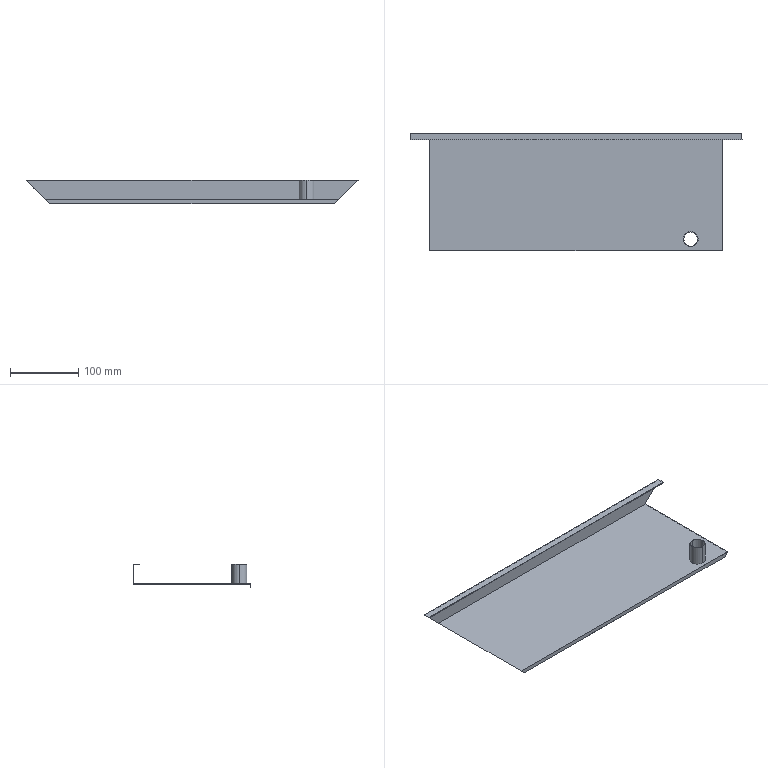Part | STEP file | 09-05 Inner side plate 2 | 1 solid | 17 faces | box 485 x 172 x 35 mm | volume 94551 mm3 | plane 13 | cylinder 4 | commonest cylinder face diameters 20 x2 22 x2
STEP:
#1=CARTESIAN_POINT('',(0.,0.,0.));
#2=DIRECTION('',(0.,0.,1.));
#3=DIRECTION('',(1.,0.,0.));
#4=AXIS2_PLACEMENT_3D('',#1,#2,#3);
#5=CARTESIAN_POINT('',(410.,6.,30.));
#6=VERTEX_POINT('',#5);
#7=CARTESIAN_POINT('',(410.,28.,30.));
#8=VERTEX_POINT('',#7);
#9=CARTESIAN_POINT('',(410.,17.,30.));
#10=DIRECTION('',(0.,0.,1.));
#11=DIRECTION('',(0.,1.,0.));
#12=AXIS2_PLACEMENT_3D('',#9,#10,#11);
#13=CIRCLE('',#12,11.);
#14=CARTESIAN_POINT('',(410.,17.,30.));
#15=DIRECTION('',(0.,0.,-1.));
#16=DIRECTION('',(0.,1.,0.));
#17=AXIS2_PLACEMENT_3D('',#14,#15,#16);
#18=CYLINDRICAL_SURFACE('',#17,11.);
#19=CARTESIAN_POINT('',(6.283,0.));
#20=DIRECTION('',(-1.,0.));
#21=VECTOR('',#20,1.);
#22=LINE('',#19,#21);
#23=(GEOMETRIC_REPRESENTATION_CONTEXT(2)PARAMETRIC_REPRESENTATION_CONTEXT()REPRESENTATION_CONTEXT('',''));
#24=DEFINITIONAL_REPRESENTATION('',(#22),#23);
#25=PCURVE('',#18,#24);
#26=CARTESIAN_POINT('',(398.868,5.868,30.));
#27=DIRECTION('',(0.,0.,1.));
#28=DIRECTION('',(1.,0.,0.));
#29=AXIS2_PLACEMENT_3D('',#26,#27,#28);
#30=PLANE('',#29);
#31=CARTESIAN_POINT('',(11.132,11.132));
#32=DIRECTION('',(0.,1.));
#33=AXIS2_PLACEMENT_2D('',#31,#32);
#34=CIRCLE('',#33,11.);
#35=(GEOMETRIC_REPRESENTATION_CONTEXT(2)PARAMETRIC_REPRESENTATION_CONTEXT()REPRESENTATION_CONTEXT('',''));
#36=DEFINITIONAL_REPRESENTATION('',(#34),#35);
#37=PCURVE('',#30,#36);
#38=SURFACE_CURVE('',#13,(#25,#37),.PCURVE_S1.);
#39=EDGE_CURVE('',#6,#8,#38,.T.);
#40=ORIENTED_EDGE('',*,*,#39,.F.);
#41=CARTESIAN_POINT('',(410.,6.,1.));
#42=VERTEX_POINT('',#41);
#43=CARTESIAN_POINT('',(410.,6.,30.));
#44=DIRECTION('',(0.,0.,-1.));
#45=VECTOR('',#44,1.);
#46=LINE('',#43,#45);
#47=CARTESIAN_POINT('',(3.142,0.));
#48=DIRECTION('',(0.,1.));
#49=VECTOR('',#48,1.);
#50=LINE('',#47,#49);
#51=(GEOMETRIC_REPRESENTATION_CONTEXT(2)PARAMETRIC_REPRESENTATION_CONTEXT()REPRESENTATION_CONTEXT('',''));
#52=DEFINITIONAL_REPRESENTATION('',(#50),#51);
#53=PCURVE('',#18,#52);
#54=CARTESIAN_POINT('',(410.,17.,30.));
#55=DIRECTION('',(0.,0.,-1.));
#56=DIRECTION('',(0.,1.,0.));
#57=AXIS2_PLACEMENT_3D('',#54,#55,#56);
#58=CYLINDRICAL_SURFACE('',#57,11.);
#59=CARTESIAN_POINT('',(3.142,0.));
#60=DIRECTION('',(0.,1.));
#61=VECTOR('',#60,1.);
#62=LINE('',#59,#61);
#63=(GEOMETRIC_REPRESENTATION_CONTEXT(2)PARAMETRIC_REPRESENTATION_CONTEXT()REPRESENTATION_CONTEXT('',''));
#64=DEFINITIONAL_REPRESENTATION('',(#62),#63);
#65=PCURVE('',#58,#64);
#66=SURFACE_CURVE('',#46,(#53,#65),.PCURVE_S1.);
#67=EDGE_CURVE('',#6,#42,#66,.T.);
#68=ORIENTED_EDGE('',*,*,#67,.T.);
#69=CARTESIAN_POINT('',(410.,28.,1.));
#70=VERTEX_POINT('',#69);
#71=CARTESIAN_POINT('',(410.,17.,1.));
#72=DIRECTION('',(0.,0.,-1.));
#73=DIRECTION('',(0.,1.,0.));
#74=AXIS2_PLACEMENT_3D('',#71,#72,#73);
#75=CIRCLE('',#74,11.);
#76=CARTESIAN_POINT('',(0.,29.));
#77=DIRECTION('',(1.,0.));
#78=VECTOR('',#77,1.);
#79=LINE('',#76,#78);
#80=(GEOMETRIC_REPRESENTATION_CONTEXT(2)PARAMETRIC_REPRESENTATION_CONTEXT()REPRESENTATION_CONTEXT('',''));
#81=DEFINITIONAL_REPRESENTATION('',(#79),#80);
#82=PCURVE('',#18,#81);
#83=CARTESIAN_POINT('',(29.,0.,1.));
#84=DIRECTION('',(0.,0.,-1.));
#85=DIRECTION('',(0.,1.,0.));
#86=AXIS2_PLACEMENT_3D('',#83,#84,#85);
#87=PLANE('',#86);
#88=CARTESIAN_POINT('',(17.,381.));
#89=DIRECTION('',(1.,0.));
#90=AXIS2_PLACEMENT_2D('',#88,#89);
#91=CIRCLE('',#90,11.);
#92=(GEOMETRIC_REPRESENTATION_CONTEXT(2)PARAMETRIC_REPRESENTATION_CONTEXT()REPRESENTATION_CONTEXT('',''));
#93=DEFINITIONAL_REPRESENTATION('',(#91),#92);
#94=PCURVE('',#87,#93);
#95=SURFACE_CURVE('',#75,(#82,#94),.PCURVE_S1.);
#96=EDGE_CURVE('',#70,#42,#95,.T.);
#97=ORIENTED_EDGE('',*,*,#96,.F.);
#98=CARTESIAN_POINT('',(410.,28.,30.));
#99=DIRECTION('',(0.,0.,-1.));
#100=VECTOR('',#99,1.);
#101=LINE('',#98,#100);
#102=CARTESIAN_POINT('',(0.,0.));
#103=DIRECTION('',(0.,1.));
#104=VECTOR('',#103,1.);
#105=LINE('',#102,#104);
#106=(GEOMETRIC_REPRESENTATION_CONTEXT(2)PARAMETRIC_REPRESENTATION_CONTEXT()REPRESENTATION_CONTEXT('',''));
#107=DEFINITIONAL_REPRESENTATION('',(#105),#106);
#108=PCURVE('',#18,#107);
#109=CARTESIAN_POINT('',(6.283,0.));
#110=DIRECTION('',(0.,1.));
#111=VECTOR('',#110,1.);
#112=LINE('',#109,#111);
#113=(GEOMETRIC_REPRESENTATION_CONTEXT(2)PARAMETRIC_REPRESENTATION_CONTEXT()REPRESENTATION_CONTEXT('',''));
#114=DEFINITIONAL_REPRESENTATION('',(#112),#113);
#115=PCURVE('',#58,#114);
#116=SURFACE_CURVE('',#101,(#108,#115),.PCURVE_S1.);
#117=EDGE_CURVE('',#8,#70,#116,.T.);
#118=ORIENTED_EDGE('',*,*,#117,.F.);
#119=EDGE_LOOP('',(#40,#68,#97,#118));
#120=FACE_BOUND('',#119,.T.);
#121=ADVANCED_FACE('',(#120),#18,.T.);
#122=CARTESIAN_POINT('',(400.,17.,30.));
#123=VERTEX_POINT('',#122);
#124=CARTESIAN_POINT('',(400.,17.,0.));
#125=VERTEX_POINT('',#124);
#126=CARTESIAN_POINT('',(400.,17.,30.));
#127=DIRECTION('',(0.,0.,-1.));
#128=VECTOR('',#127,1.);
#129=LINE('',#126,#128);
#130=CARTESIAN_POINT('',(410.,17.,30.));
#131=DIRECTION('',(0.,0.,-1.));
#132=DIRECTION('',(-1.,0.,0.));
#133=AXIS2_PLACEMENT_3D('',#130,#131,#132);
#134=CYLINDRICAL_SURFACE('',#133,10.);
#135=CARTESIAN_POINT('',(6.283,0.));
#136=DIRECTION('',(0.,1.));
#137=VECTOR('',#136,1.);
#138=LINE('',#135,#137);
#139=(GEOMETRIC_REPRESENTATION_CONTEXT(2)PARAMETRIC_REPRESENTATION_CONTEXT()REPRESENTATION_CONTEXT('',''));
#140=DEFINITIONAL_REPRESENTATION('',(#138),#139);
#141=PCURVE('',#134,#140);
#142=CARTESIAN_POINT('',(410.,17.,30.));
#143=DIRECTION('',(0.,0.,-1.));
#144=DIRECTION('',(-1.,0.,0.));
#145=AXIS2_PLACEMENT_3D('',#142,#143,#144);
#146=CYLINDRICAL_SURFACE('',#145,10.);
#147=CARTESIAN_POINT('',(0.,0.));
#148=DIRECTION('',(0.,1.));
#149=VECTOR('',#148,1.);
#150=LINE('',#147,#149);
#151=(GEOMETRIC_REPRESENTATION_CONTEXT(2)PARAMETRIC_REPRESENTATION_CONTEXT()REPRESENTATION_CONTEXT('',''));
#152=DEFINITIONAL_REPRESENTATION('',(#150),#151);
#153=PCURVE('',#146,#152);
#154=SURFACE_CURVE('',#129,(#141,#153),.PCURVE_S1.);
#155=EDGE_CURVE('',#123,#125,#154,.T.);
#156=ORIENTED_EDGE('',*,*,#155,.T.);
#157=CARTESIAN_POINT('',(420.,17.,0.));
#158=VERTEX_POINT('',#157);
#159=CARTESIAN_POINT('',(410.,17.,0.));
#160=DIRECTION('',(0.,0.,-1.));
#161=DIRECTION('',(-1.,0.,0.));
#162=AXIS2_PLACEMENT_3D('',#159,#160,#161);
#163=CIRCLE('',#162,10.);
#164=CARTESIAN_POINT('',(0.,30.));
#165=DIRECTION('',(1.,0.));
#166=VECTOR('',#165,1.);
#167=LINE('',#164,#166);
#168=(GEOMETRIC_REPRESENTATION_CONTEXT(2)PARAMETRIC_REPRESENTATION_CONTEXT()REPRESENTATION_CONTEXT('',''));
#169=DEFINITIONAL_REPRESENTATION('',(#167),#168);
#170=PCURVE('',#134,#169);
#171=CARTESIAN_POINT('',(30.,172.,0.));
#172=DIRECTION('',(0.,0.,1.));
#173=DIRECTION('',(0.,-1.,0.));
#174=AXIS2_PLACEMENT_3D('',#171,#172,#173);
#175=PLANE('',#174);
#176=CARTESIAN_POINT('',(155.,370.));
#177=CARTESIAN_POINT('',(137.679,370.));
#178=CARTESIAN_POINT('',(146.34,385.));
#179=CARTESIAN_POINT('',(155.,400.));
#180=CARTESIAN_POINT('',(163.66,385.));
#181=CARTESIAN_POINT('',(172.321,370.));
#182=CARTESIAN_POINT('',(155.,370.));
#183=(BOUNDED_CURVE()B_SPLINE_CURVE(2,(#176,#177,#178,#179,#180,#181,#182),.UNSPECIFIED.,.T.,.F.)B_SPLINE_CURVE_WITH_KNOTS((1,2,2,2,2,1),(-2.094,0.,2.094,4.189,6.283,8.378),.UNSPECIFIED.)CURVE()GEOMETRIC_REPRESENTATION_ITEM()RATIONAL_B_SPLINE_CURVE((1.,0.5,1.,0.5,1.,0.5,1.))REPRESENTATION_ITEM(''));
#184=(GEOMETRIC_REPRESENTATION_CONTEXT(2)PARAMETRIC_REPRESENTATION_CONTEXT()REPRESENTATION_CONTEXT('',''));
#185=DEFINITIONAL_REPRESENTATION('',(#183),#184);
#186=PCURVE('',#175,#185);
#187=SURFACE_CURVE('',#163,(#170,#186),.PCURVE_S1.);
#188=EDGE_CURVE('',#158,#125,#187,.T.);
#189=ORIENTED_EDGE('',*,*,#188,.F.);
#190=CARTESIAN_POINT('',(420.,17.,30.));
#191=VERTEX_POINT('',#190);
#192=CARTESIAN_POINT('',(420.,17.,30.));
#193=DIRECTION('',(0.,0.,-1.));
#194=VECTOR('',#193,1.);
#195=LINE('',#192,#194);
#196=CARTESIAN_POINT('',(3.142,0.));
#197=DIRECTION('',(0.,1.));
#198=VECTOR('',#197,1.);
#199=LINE('',#196,#198);
#200=(GEOMETRIC_REPRESENTATION_CONTEXT(2)PARAMETRIC_REPRESENTATION_CONTEXT()REPRESENTATION_CONTEXT('',''));
#201=DEFINITIONAL_REPRESENTATION('',(#199),#200);
#202=PCURVE('',#134,#201);
#203=CARTESIAN_POINT('',(3.142,0.));
#204=DIRECTION('',(0.,1.));
#205=VECTOR('',#204,1.);
#206=LINE('',#203,#205);
#207=(GEOMETRIC_REPRESENTATION_CONTEXT(2)PARAMETRIC_REPRESENTATION_CONTEXT()REPRESENTATION_CONTEXT('',''));
#208=DEFINITIONAL_REPRESENTATION('',(#206),#207);
#209=PCURVE('',#146,#208);
#210=SURFACE_CURVE('',#195,(#202,#209),.PCURVE_S1.);
#211=EDGE_CURVE('',#191,#158,#210,.T.);
#212=ORIENTED_EDGE('',*,*,#211,.F.);
#213=CARTESIAN_POINT('',(410.,17.,30.));
#214=DIRECTION('',(0.,0.,-1.));
#215=DIRECTION('',(-1.,0.,0.));
#216=AXIS2_PLACEMENT_3D('',#213,#214,#215);
#217=CIRCLE('',#216,10.);
#218=CARTESIAN_POINT('',(0.,0.));
#219=DIRECTION('',(1.,0.));
#220=VECTOR('',#219,1.);
#221=LINE('',#218,#220);
#222=(GEOMETRIC_REPRESENTATION_CONTEXT(2)PARAMETRIC_REPRESENTATION_CONTEXT()REPRESENTATION_CONTEXT('',''));
#223=DEFINITIONAL_REPRESENTATION('',(#221),#222);
#224=PCURVE('',#134,#223);
#225=CARTESIAN_POINT('',(1.132,11.132));
#226=CARTESIAN_POINT('',(1.132,28.453));
#227=CARTESIAN_POINT('',(16.132,19.792));
#228=CARTESIAN_POINT('',(31.132,11.132));
#229=CARTESIAN_POINT('',(16.132,2.472));
#230=CARTESIAN_POINT('',(1.132,-6.189));
#231=CARTESIAN_POINT('',(1.132,11.132));
#232=(BOUNDED_CURVE()B_SPLINE_CURVE(2,(#225,#226,#227,#228,#229,#230,#231),.UNSPECIFIED.,.T.,.F.)B_SPLINE_CURVE_WITH_KNOTS((1,2,2,2,2,1),(-2.094,0.,2.094,4.189,6.283,8.378),.UNSPECIFIED.)CURVE()GEOMETRIC_REPRESENTATION_ITEM()RATIONAL_B_SPLINE_CURVE((1.,0.5,1.,0.5,1.,0.5,1.))REPRESENTATION_ITEM(''));
#233=(GEOMETRIC_REPRESENTATION_CONTEXT(2)PARAMETRIC_REPRESENTATION_CONTEXT()REPRESENTATION_CONTEXT('',''));
#234=DEFINITIONAL_REPRESENTATION('',(#232),#233);
#235=PCURVE('',#30,#234);
#236=SURFACE_CURVE('',#217,(#224,#235),.PCURVE_S1.);
#237=EDGE_CURVE('',#191,#123,#236,.T.);
#238=ORIENTED_EDGE('',*,*,#237,.T.);
#239=EDGE_LOOP('',(#156,#189,#212,#238));
#240=FACE_BOUND('',#239,.F.);
#241=ADVANCED_FACE('',(#240),#134,.F.);
#242=ORIENTED_EDGE('',*,*,#67,.F.);
#243=CARTESIAN_POINT('',(410.,17.,30.));
#244=DIRECTION('',(0.,0.,1.));
#245=DIRECTION('',(0.,1.,0.));
#246=AXIS2_PLACEMENT_3D('',#243,#244,#245);
#247=CIRCLE('',#246,11.);
#248=CARTESIAN_POINT('',(6.283,0.));
#249=DIRECTION('',(-1.,0.));
#250=VECTOR('',#249,1.);
#251=LINE('',#248,#250);
#252=(GEOMETRIC_REPRESENTATION_CONTEXT(2)PARAMETRIC_REPRESENTATION_CONTEXT()REPRESENTATION_CONTEXT('',''));
#253=DEFINITIONAL_REPRESENTATION('',(#251),#252);
#254=PCURVE('',#58,#253);
#255=CARTESIAN_POINT('',(11.132,11.132));
#256=DIRECTION('',(0.,1.));
#257=AXIS2_PLACEMENT_2D('',#255,#256);
#258=CIRCLE('',#257,11.);
#259=(GEOMETRIC_REPRESENTATION_CONTEXT(2)PARAMETRIC_REPRESENTATION_CONTEXT()REPRESENTATION_CONTEXT('',''));
#260=DEFINITIONAL_REPRESENTATION('',(#258),#259);
#261=PCURVE('',#30,#260);
#262=SURFACE_CURVE('',#247,(#254,#261),.PCURVE_S1.);
#263=EDGE_CURVE('',#8,#6,#262,.T.);
#264=ORIENTED_EDGE('',*,*,#263,.F.);
#265=ORIENTED_EDGE('',*,*,#117,.T.);
#266=CARTESIAN_POINT('',(410.,17.,1.));
#267=DIRECTION('',(0.,0.,-1.));
#268=DIRECTION('',(0.,1.,0.));
#269=AXIS2_PLACEMENT_3D('',#266,#267,#268);
#270=CIRCLE('',#269,11.);
#271=CARTESIAN_POINT('',(0.,29.));
#272=DIRECTION('',(1.,0.));
#273=VECTOR('',#272,1.);
#274=LINE('',#271,#273);
#275=(GEOMETRIC_REPRESENTATION_CONTEXT(2)PARAMETRIC_REPRESENTATION_CONTEXT()REPRESENTATION_CONTEXT('',''));
#276=DEFINITIONAL_REPRESENTATION('',(#274),#275);
#277=PCURVE('',#58,#276);
#278=CARTESIAN_POINT('',(17.,381.));
#279=DIRECTION('',(1.,0.));
#280=AXIS2_PLACEMENT_2D('',#278,#279);
#281=CIRCLE('',#280,11.);
#282=(GEOMETRIC_REPRESENTATION_CONTEXT(2)PARAMETRIC_REPRESENTATION_CONTEXT()REPRESENTATION_CONTEXT('',''));
#283=DEFINITIONAL_REPRESENTATION('',(#281),#282);
#284=PCURVE('',#87,#283);
#285=SURFACE_CURVE('',#270,(#277,#284),.PCURVE_S1.);
#286=EDGE_CURVE('',#42,#70,#285,.T.);
#287=ORIENTED_EDGE('',*,*,#286,.F.);
#288=EDGE_LOOP('',(#242,#264,#265,#287));
#289=FACE_BOUND('',#288,.T.);
#290=ADVANCED_FACE('',(#289),#58,.T.);
#291=CARTESIAN_POINT('',(410.,17.,30.));
#292=DIRECTION('',(0.,0.,-1.));
#293=DIRECTION('',(-1.,0.,0.));
#294=AXIS2_PLACEMENT_3D('',#291,#292,#293);
#295=CIRCLE('',#294,10.);
#296=CARTESIAN_POINT('',(1.132,11.132));
#297=CARTESIAN_POINT('',(1.132,28.453));
#298=CARTESIAN_POINT('',(16.132,19.792));
#299=CARTESIAN_POINT('',(31.132,11.132));
#300=CARTESIAN_POINT('',(16.132,2.472));
#301=CARTESIAN_POINT('',(1.132,-6.189));
#302=CARTESIAN_POINT('',(1.132,11.132));
#303=(BOUNDED_CURVE()B_SPLINE_CURVE(2,(#296,#297,#298,#299,#300,#301,#302),.UNSPECIFIED.,.T.,.F.)B_SPLINE_CURVE_WITH_KNOTS((1,2,2,2,2,1),(-2.094,0.,2.094,4.189,6.283,8.378),.UNSPECIFIED.)CURVE()GEOMETRIC_REPRESENTATION_ITEM()RATIONAL_B_SPLINE_CURVE((1.,0.5,1.,0.5,1.,0.5,1.))REPRESENTATION_ITEM(''));
#304=(GEOMETRIC_REPRESENTATION_CONTEXT(2)PARAMETRIC_REPRESENTATION_CONTEXT()REPRESENTATION_CONTEXT('',''));
#305=DEFINITIONAL_REPRESENTATION('',(#303),#304);
#306=PCURVE('',#30,#305);
#307=CARTESIAN_POINT('',(0.,0.));
#308=DIRECTION('',(1.,0.));
#309=VECTOR('',#308,1.);
#310=LINE('',#307,#309);
#311=(GEOMETRIC_REPRESENTATION_CONTEXT(2)PARAMETRIC_REPRESENTATION_CONTEXT()REPRESENTATION_CONTEXT('',''));
#312=DEFINITIONAL_REPRESENTATION('',(#310),#311);
#313=PCURVE('',#146,#312);
#314=SURFACE_CURVE('',#295,(#306,#313),.PCURVE_S1.);
#315=EDGE_CURVE('',#123,#191,#314,.T.);
#316=ORIENTED_EDGE('',*,*,#315,.T.);
#317=ORIENTED_EDGE('',*,*,#237,.T.);
#318=EDGE_LOOP('',(#316,#317));
#319=FACE_BOUND('',#318,.T.);
#320=ORIENTED_EDGE('',*,*,#263,.T.);
#321=ORIENTED_EDGE('',*,*,#39,.T.);
#322=EDGE_LOOP('',(#320,#321));
#323=FACE_BOUND('',#322,.T.);
#324=ADVANCED_FACE('',(#319,#323),#30,.T.);
#325=ORIENTED_EDGE('',*,*,#96,.T.);
#326=ORIENTED_EDGE('',*,*,#286,.T.);
#327=EDGE_LOOP('',(#325,#326));
#328=FACE_BOUND('',#327,.T.);
#329=CARTESIAN_POINT('',(456.,171.,1.));
#330=VERTEX_POINT('',#329);
#331=CARTESIAN_POINT('',(456.,0.,1.));
#332=VERTEX_POINT('',#331);
#333=CARTESIAN_POINT('',(456.,85.5,1.));
#334=DIRECTION('',(0.,-1.,0.));
#335=VECTOR('',#334,1.);
#336=LINE('',#333,#335);
#337=CARTESIAN_POINT('',(85.5,427.));
#338=DIRECTION('',(-1.,0.));
#339=VECTOR('',#338,1.);
#340=LINE('',#337,#339);
#341=(GEOMETRIC_REPRESENTATION_CONTEXT(2)PARAMETRIC_REPRESENTATION_CONTEXT()REPRESENTATION_CONTEXT('',''));
#342=DEFINITIONAL_REPRESENTATION('',(#340),#341);
#343=PCURVE('',#87,#342);
#344=CARTESIAN_POINT('',(450.,0.,-5.));
#345=DIRECTION('',(-0.7071,0.,0.7071));
#346=DIRECTION('',(0.7071,0.,0.7071));
#347=AXIS2_PLACEMENT_3D('',#344,#345,#346);
#348=PLANE('',#347);
#349=CARTESIAN_POINT('',(8.485,85.5));
#350=DIRECTION('',(0.,-1.));
#351=VECTOR('',#350,1.);
#352=LINE('',#349,#351);
#353=(GEOMETRIC_REPRESENTATION_CONTEXT(2)PARAMETRIC_REPRESENTATION_CONTEXT()REPRESENTATION_CONTEXT('',''));
#354=DEFINITIONAL_REPRESENTATION('',(#352),#353);
#355=PCURVE('',#348,#354);
#356=SURFACE_CURVE('',#336,(#343,#355),.PCURVE_S1.);
#357=EDGE_CURVE('',#330,#332,#356,.T.);
#358=ORIENTED_EDGE('',*,*,#357,.F.);
#359=CARTESIAN_POINT('',(29.,171.,1.));
#360=VERTEX_POINT('',#359);
#361=CARTESIAN_POINT('',(242.5,171.,1.));
#362=DIRECTION('',(1.,0.,0.));
#363=VECTOR('',#362,1.);
#364=LINE('',#361,#363);
#365=CARTESIAN_POINT('',(171.,213.5));
#366=DIRECTION('',(0.,1.));
#367=VECTOR('',#366,1.);
#368=LINE('',#365,#367);
#369=(GEOMETRIC_REPRESENTATION_CONTEXT(2)PARAMETRIC_REPRESENTATION_CONTEXT()REPRESENTATION_CONTEXT('',''));
#370=DEFINITIONAL_REPRESENTATION('',(#368),#369);
#371=PCURVE('',#87,#370);
#372=CARTESIAN_POINT('',(-1.898,171.,1.));
#373=DIRECTION('',(0.,1.,0.));
#374=DIRECTION('',(0.,0.,1.));
#375=AXIS2_PLACEMENT_3D('',#372,#373,#374);
#376=PLANE('',#375);
#377=CARTESIAN_POINT('',(0.,244.398));
#378=DIRECTION('',(0.,1.));
#379=VECTOR('',#378,1.);
#380=LINE('',#377,#379);
#381=(GEOMETRIC_REPRESENTATION_CONTEXT(2)PARAMETRIC_REPRESENTATION_CONTEXT()REPRESENTATION_CONTEXT('',''));
#382=DEFINITIONAL_REPRESENTATION('',(#380),#381);
#383=PCURVE('',#376,#382);
#384=SURFACE_CURVE('',#364,(#371,#383),.PCURVE_S1.);
#385=EDGE_CURVE('',#360,#330,#384,.T.);
#386=ORIENTED_EDGE('',*,*,#385,.F.);
#387=CARTESIAN_POINT('',(29.,0.,1.));
#388=VERTEX_POINT('',#387);
#389=CARTESIAN_POINT('',(29.,85.5,1.));
#390=DIRECTION('',(0.,1.,0.));
#391=VECTOR('',#390,1.);
#392=LINE('',#389,#391);
#393=CARTESIAN_POINT('',(85.5,0.));
#394=DIRECTION('',(1.,0.));
#395=VECTOR('',#394,1.);
#396=LINE('',#393,#395);
#397=(GEOMETRIC_REPRESENTATION_CONTEXT(2)PARAMETRIC_REPRESENTATION_CONTEXT()REPRESENTATION_CONTEXT('',''));
#398=DEFINITIONAL_REPRESENTATION('',(#396),#397);
#399=PCURVE('',#87,#398);
#400=CARTESIAN_POINT('',(0.,0.,30.));
#401=DIRECTION('',(0.7071,0.,0.7071));
#402=DIRECTION('',(0.7071,0.,-0.7071));
#403=AXIS2_PLACEMENT_3D('',#400,#401,#402);
#404=PLANE('',#403);
#405=CARTESIAN_POINT('',(41.012,85.5));
#406=DIRECTION('',(0.,1.));
#407=VECTOR('',#406,1.);
#408=LINE('',#405,#407);
#409=(GEOMETRIC_REPRESENTATION_CONTEXT(2)PARAMETRIC_REPRESENTATION_CONTEXT()REPRESENTATION_CONTEXT('',''));
#410=DEFINITIONAL_REPRESENTATION('',(#408),#409);
#411=PCURVE('',#404,#410);
#412=SURFACE_CURVE('',#392,(#399,#411),.PCURVE_S1.);
#413=EDGE_CURVE('',#388,#360,#412,.T.);
#414=ORIENTED_EDGE('',*,*,#413,.F.);
#415=CARTESIAN_POINT('',(242.5,0.,1.));
#416=DIRECTION('',(-1.,0.,0.));
#417=VECTOR('',#416,1.);
#418=LINE('',#415,#417);
#419=CARTESIAN_POINT('',(0.,213.5));
#420=DIRECTION('',(0.,-1.));
#421=VECTOR('',#420,1.);
#422=LINE('',#419,#421);
#423=(GEOMETRIC_REPRESENTATION_CONTEXT(2)PARAMETRIC_REPRESENTATION_CONTEXT()REPRESENTATION_CONTEXT('',''));
#424=DEFINITIONAL_REPRESENTATION('',(#422),#423);
#425=PCURVE('',#87,#424);
#426=CARTESIAN_POINT('',(26.438,0.,-5.));
#427=DIRECTION('',(0.,1.,0.));
#428=DIRECTION('',(0.,0.,1.));
#429=AXIS2_PLACEMENT_3D('',#426,#427,#428);
#430=PLANE('',#429);
#431=CARTESIAN_POINT('',(6.,216.062));
#432=DIRECTION('',(0.,-1.));
#433=VECTOR('',#432,1.);
#434=LINE('',#431,#433);
#435=(GEOMETRIC_REPRESENTATION_CONTEXT(2)PARAMETRIC_REPRESENTATION_CONTEXT()REPRESENTATION_CONTEXT('',''));
#436=DEFINITIONAL_REPRESENTATION('',(#434),#435);
#437=PCURVE('',#430,#436);
#438=SURFACE_CURVE('',#418,(#425,#437),.PCURVE_S1.);
#439=EDGE_CURVE('',#332,#388,#438,.T.);
#440=ORIENTED_EDGE('',*,*,#439,.F.);
#441=EDGE_LOOP('',(#358,#386,#414,#440));
#442=FACE_BOUND('',#441,.T.);
#443=ADVANCED_FACE('',(#328,#442),#87,.F.);
#444=CARTESIAN_POINT('',(410.,17.,0.));
#445=DIRECTION('',(0.,0.,-1.));
#446=DIRECTION('',(-1.,0.,0.));
#447=AXIS2_PLACEMENT_3D('',#444,#445,#446);
#448=CIRCLE('',#447,10.);
#449=CARTESIAN_POINT('',(0.,30.));
#450=DIRECTION('',(1.,0.));
#451=VECTOR('',#450,1.);
#452=LINE('',#449,#451);
#453=(GEOMETRIC_REPRESENTATION_CONTEXT(2)PARAMETRIC_REPRESENTATION_CONTEXT()REPRESENTATION_CONTEXT('',''));
#454=DEFINITIONAL_REPRESENTATION('',(#452),#453);
#455=PCURVE('',#146,#454);
#456=CARTESIAN_POINT('',(155.,370.));
#457=CARTESIAN_POINT('',(137.679,370.));
#458=CARTESIAN_POINT('',(146.34,385.));
#459=CARTESIAN_POINT('',(155.,400.));
#460=CARTESIAN_POINT('',(163.66,385.));
#461=CARTESIAN_POINT('',(172.321,370.));
#462=CARTESIAN_POINT('',(155.,370.));
#463=(BOUNDED_CURVE()B_SPLINE_CURVE(2,(#456,#457,#458,#459,#460,#461,#462),.UNSPECIFIED.,.T.,.F.)B_SPLINE_CURVE_WITH_KNOTS((1,2,2,2,2,1),(-2.094,0.,2.094,4.189,6.283,8.378),.UNSPECIFIED.)CURVE()GEOMETRIC_REPRESENTATION_ITEM()RATIONAL_B_SPLINE_CURVE((1.,0.5,1.,0.5,1.,0.5,1.))REPRESENTATION_ITEM(''));
#464=(GEOMETRIC_REPRESENTATION_CONTEXT(2)PARAMETRIC_REPRESENTATION_CONTEXT()REPRESENTATION_CONTEXT('',''));
#465=DEFINITIONAL_REPRESENTATION('',(#463),#464);
#466=PCURVE('',#175,#465);
#467=SURFACE_CURVE('',#448,(#455,#466),.PCURVE_S1.);
#468=EDGE_CURVE('',#125,#158,#467,.T.);
#469=ORIENTED_EDGE('',*,*,#468,.F.);
#470=ORIENTED_EDGE('',*,*,#155,.F.);
#471=ORIENTED_EDGE('',*,*,#315,.T.);
#472=ORIENTED_EDGE('',*,*,#211,.T.);
#473=EDGE_LOOP('',(#469,#470,#471,#472));
#474=FACE_BOUND('',#473,.F.);
#475=ADVANCED_FACE('',(#474),#146,.F.);
#476=CARTESIAN_POINT('',(450.,0.,-5.));
#477=VERTEX_POINT('',#476);
#478=CARTESIAN_POINT('',(450.,0.,-5.));
#479=DIRECTION('',(-0.7071,0.,-0.7071));
#480=VECTOR('',#479,1.);
#481=LINE('',#478,#480);
#482=CARTESIAN_POINT('',(0.,423.562));
#483=DIRECTION('',(-0.7071,-0.7071));
#484=VECTOR('',#483,1.);
#485=LINE('',#482,#484);
#486=(GEOMETRIC_REPRESENTATION_CONTEXT(2)PARAMETRIC_REPRESENTATION_CONTEXT()REPRESENTATION_CONTEXT('',''));
#487=DEFINITIONAL_REPRESENTATION('',(#485),#486);
#488=PCURVE('',#430,#487);
#489=CARTESIAN_POINT('',(0.,0.));
#490=DIRECTION('',(-1.,0.));
#491=VECTOR('',#490,1.);
#492=LINE('',#489,#491);
#493=(GEOMETRIC_REPRESENTATION_CONTEXT(2)PARAMETRIC_REPRESENTATION_CONTEXT()REPRESENTATION_CONTEXT('',''));
#494=DEFINITIONAL_REPRESENTATION('',(#492),#493);
#495=PCURVE('',#348,#494);
#496=SURFACE_CURVE('',#481,(#488,#495),.PCURVE_S1.);
#497=EDGE_CURVE('',#332,#477,#496,.T.);
#498=ORIENTED_EDGE('',*,*,#497,.F.);
#499=ORIENTED_EDGE('',*,*,#439,.T.);
#500=CARTESIAN_POINT('',(35.,0.,-5.));
#501=VERTEX_POINT('',#500);
#502=CARTESIAN_POINT('',(0.,0.,30.));
#503=DIRECTION('',(-0.7071,0.,0.7071));
#504=VECTOR('',#503,1.);
#505=LINE('',#502,#504);
#506=CARTESIAN_POINT('',(35.,-26.438));
#507=DIRECTION('',(0.7071,-0.7071));
#508=VECTOR('',#507,1.);
#509=LINE('',#506,#508);
#510=(GEOMETRIC_REPRESENTATION_CONTEXT(2)PARAMETRIC_REPRESENTATION_CONTEXT()REPRESENTATION_CONTEXT('',''));
#511=DEFINITIONAL_REPRESENTATION('',(#509),#510);
#512=PCURVE('',#430,#511);
#513=CARTESIAN_POINT('',(0.,0.));
#514=DIRECTION('',(-1.,0.));
#515=VECTOR('',#514,1.);
#516=LINE('',#513,#515);
#517=(GEOMETRIC_REPRESENTATION_CONTEXT(2)PARAMETRIC_REPRESENTATION_CONTEXT()REPRESENTATION_CONTEXT('',''));
#518=DEFINITIONAL_REPRESENTATION('',(#516),#517);
#519=PCURVE('',#404,#518);
#520=SURFACE_CURVE('',#505,(#512,#519),.PCURVE_S1.);
#521=EDGE_CURVE('',#501,#388,#520,.T.);
#522=ORIENTED_EDGE('',*,*,#521,.F.);
#523=CARTESIAN_POINT('',(242.5,0.,-5.));
#524=DIRECTION('',(-1.,0.,0.));
#525=VECTOR('',#524,1.);
#526=LINE('',#523,#525);
#527=CARTESIAN_POINT('',(0.,216.062));
#528=DIRECTION('',(0.,-1.));
#529=VECTOR('',#528,1.);
#530=LINE('',#527,#529);
#531=(GEOMETRIC_REPRESENTATION_CONTEXT(2)PARAMETRIC_REPRESENTATION_CONTEXT()REPRESENTATION_CONTEXT('',''));
#532=DEFINITIONAL_REPRESENTATION('',(#530),#531);
#533=PCURVE('',#430,#532);
#534=CARTESIAN_POINT('',(35.,0.,-5.));
#535=DIRECTION('',(0.,0.,1.));
#536=DIRECTION('',(1.,0.,0.));
#537=AXIS2_PLACEMENT_3D('',#534,#535,#536);
#538=PLANE('',#537);
#539=CARTESIAN_POINT('',(207.5,0.));
#540=DIRECTION('',(-1.,0.));
#541=VECTOR('',#540,1.);
#542=LINE('',#539,#541);
#543=(GEOMETRIC_REPRESENTATION_CONTEXT(2)PARAMETRIC_REPRESENTATION_CONTEXT()REPRESENTATION_CONTEXT('',''));
#544=DEFINITIONAL_REPRESENTATION('',(#542),#543);
#545=PCURVE('',#538,#544);
#546=SURFACE_CURVE('',#526,(#533,#545),.PCURVE_S1.);
#547=EDGE_CURVE('',#477,#501,#546,.T.);
#548=ORIENTED_EDGE('',*,*,#547,.F.);
#549=EDGE_LOOP('',(#498,#499,#522,#548));
#550=FACE_BOUND('',#549,.T.);
#551=ADVANCED_FACE('',(#550),#430,.F.);
#552=CARTESIAN_POINT('',(485.,172.,30.));
#553=VERTEX_POINT('',#552);
#554=CARTESIAN_POINT('',(455.,172.,0.000000001));
#555=VERTEX_POINT('',#554);
#556=CARTESIAN_POINT('',(467.5,172.,12.5));
#557=DIRECTION('',(-0.7071,0.,-0.7071));
#558=VECTOR('',#557,1.);
#559=LINE('',#556,#558);
#560=CARTESIAN_POINT('',(24.749,172.));
#561=DIRECTION('',(-1.,0.));
#562=VECTOR('',#561,1.);
#563=LINE('',#560,#562);
#564=(GEOMETRIC_REPRESENTATION_CONTEXT(2)PARAMETRIC_REPRESENTATION_CONTEXT()REPRESENTATION_CONTEXT('',''));
#565=DEFINITIONAL_REPRESENTATION('',(#563),#564);
#566=PCURVE('',#348,#565);
#567=CARTESIAN_POINT('',(-2.91,172.,30.));
#568=DIRECTION('',(0.,-1.,0.));
#569=DIRECTION('',(0.,0.,-1.));
#570=AXIS2_PLACEMENT_3D('',#567,#568,#569);
#571=PLANE('',#570);
#572=CARTESIAN_POINT('',(17.5,470.41));
#573=DIRECTION('',(0.7071,-0.7071));
#574=VECTOR('',#573,1.);
#575=LINE('',#572,#574);
#576=(GEOMETRIC_REPRESENTATION_CONTEXT(2)PARAMETRIC_REPRESENTATION_CONTEXT()REPRESENTATION_CONTEXT('',''));
#577=DEFINITIONAL_REPRESENTATION('',(#575),#576);
#578=PCURVE('',#571,#577);
#579=SURFACE_CURVE('',#559,(#566,#578),.PCURVE_S1.);
#580=EDGE_CURVE('',#553,#555,#579,.T.);
#581=ORIENTED_EDGE('',*,*,#580,.F.);
#582=CARTESIAN_POINT('',(485.,162.,30.));
#583=VERTEX_POINT('',#582);
#584=CARTESIAN_POINT('',(485.,86.,30.));
#585=DIRECTION('',(0.,1.,0.));
#586=VECTOR('',#585,1.);
#587=LINE('',#584,#586);
#588=CARTESIAN_POINT('',(49.497,86.));
#589=DIRECTION('',(0.,1.));
#590=VECTOR('',#589,1.);
#591=LINE('',#588,#590);
#592=(GEOMETRIC_REPRESENTATION_CONTEXT(2)PARAMETRIC_REPRESENTATION_CONTEXT()REPRESENTATION_CONTEXT('',''));
#593=DEFINITIONAL_REPRESENTATION('',(#591),#592);
#594=PCURVE('',#348,#593);
#595=CARTESIAN_POINT('',(0.,162.,30.));
#596=DIRECTION('',(0.,0.,-1.));
#597=DIRECTION('',(0.,1.,0.));
#598=AXIS2_PLACEMENT_3D('',#595,#596,#597);
#599=PLANE('',#598);
#600=CARTESIAN_POINT('',(-76.,485.));
#601=DIRECTION('',(1.,0.));
#602=VECTOR('',#601,1.);
#603=LINE('',#600,#602);
#604=(GEOMETRIC_REPRESENTATION_CONTEXT(2)PARAMETRIC_REPRESENTATION_CONTEXT()REPRESENTATION_CONTEXT('',''));
#605=DEFINITIONAL_REPRESENTATION('',(#603),#604);
#606=PCURVE('',#599,#605);
#607=SURFACE_CURVE('',#587,(#594,#606),.PCURVE_S1.);
#608=EDGE_CURVE('',#583,#553,#607,.T.);
#609=ORIENTED_EDGE('',*,*,#608,.F.);
#610=CARTESIAN_POINT('',(484.,162.,29.));
#611=VERTEX_POINT('',#610);
#612=CARTESIAN_POINT('',(450.,162.,-5.));
#613=DIRECTION('',(-0.7071,0.,-0.7071));
#614=VECTOR('',#613,1.);
#615=LINE('',#612,#614);
#616=CARTESIAN_POINT('',(0.,162.));
#617=DIRECTION('',(-1.,0.));
#618=VECTOR('',#617,1.);
#619=LINE('',#616,#618);
#620=(GEOMETRIC_REPRESENTATION_CONTEXT(2)PARAMETRIC_REPRESENTATION_CONTEXT()REPRESENTATION_CONTEXT('',''));
#621=DEFINITIONAL_REPRESENTATION('',(#619),#620);
#622=PCURVE('',#348,#621);
#623=CARTESIAN_POINT('',(-2.91,162.,29.));
#624=DIRECTION('',(0.,1.,0.));
#625=DIRECTION('',(0.,0.,1.));
#626=AXIS2_PLACEMENT_3D('',#623,#624,#625);
#627=PLANE('',#626);
#628=CARTESIAN_POINT('',(-34.,452.91));
#629=DIRECTION('',(-0.7071,-0.7071));
#630=VECTOR('',#629,1.);
#631=LINE('',#628,#630);
#632=(GEOMETRIC_REPRESENTATION_CONTEXT(2)PARAMETRIC_REPRESENTATION_CONTEXT()REPRESENTATION_CONTEXT('',''));
#633=DEFINITIONAL_REPRESENTATION('',(#631),#632);
#634=PCURVE('',#627,#633);
#635=SURFACE_CURVE('',#615,(#622,#634),.PCURVE_S1.);
#636=EDGE_CURVE('',#583,#611,#635,.T.);
#637=ORIENTED_EDGE('',*,*,#636,.T.);
#638=CARTESIAN_POINT('',(484.,171.,29.));
#639=VERTEX_POINT('',#638);
#640=CARTESIAN_POINT('',(484.,86.,29.));
#641=DIRECTION('',(0.,-1.,0.));
#642=VECTOR('',#641,1.);
#643=LINE('',#640,#642);
#644=CARTESIAN_POINT('',(48.083,86.));
#645=DIRECTION('',(0.,-1.));
#646=VECTOR('',#645,1.);
#647=LINE('',#644,#646);
#648=(GEOMETRIC_REPRESENTATION_CONTEXT(2)PARAMETRIC_REPRESENTATION_CONTEXT()REPRESENTATION_CONTEXT('',''));
#649=DEFINITIONAL_REPRESENTATION('',(#647),#648);
#650=PCURVE('',#348,#649);
#651=CARTESIAN_POINT('',(1.,162.,29.));
#652=DIRECTION('',(0.,0.,1.));
#653=DIRECTION('',(1.,0.,0.));
#654=AXIS2_PLACEMENT_3D('',#651,#652,#653);
#655=PLANE('',#654);
#656=CARTESIAN_POINT('',(483.,-76.));
#657=DIRECTION('',(0.,-1.));
#658=VECTOR('',#657,1.);
#659=LINE('',#656,#658);
#660=(GEOMETRIC_REPRESENTATION_CONTEXT(2)PARAMETRIC_REPRESENTATION_CONTEXT()REPRESENTATION_CONTEXT('',''));
#661=DEFINITIONAL_REPRESENTATION('',(#659),#660);
#662=PCURVE('',#655,#661);
#663=SURFACE_CURVE('',#643,(#650,#662),.PCURVE_S1.);
#664=EDGE_CURVE('',#639,#611,#663,.T.);
#665=ORIENTED_EDGE('',*,*,#664,.F.);
#666=CARTESIAN_POINT('',(467.5,171.,12.5));
#667=DIRECTION('',(0.7071,0.,0.7071));
#668=VECTOR('',#667,1.);
#669=LINE('',#666,#668);
#670=CARTESIAN_POINT('',(24.749,171.));
#671=DIRECTION('',(1.,0.));
#672=VECTOR('',#671,1.);
#673=LINE('',#670,#672);
#674=(GEOMETRIC_REPRESENTATION_CONTEXT(2)PARAMETRIC_REPRESENTATION_CONTEXT()REPRESENTATION_CONTEXT('',''));
#675=DEFINITIONAL_REPRESENTATION('',(#673),#674);
#676=PCURVE('',#348,#675);
#677=CARTESIAN_POINT('',(11.5,469.398));
#678=DIRECTION('',(0.7071,0.7071));
#679=VECTOR('',#678,1.);
#680=LINE('',#677,#679);
#681=(GEOMETRIC_REPRESENTATION_CONTEXT(2)PARAMETRIC_REPRESENTATION_CONTEXT()REPRESENTATION_CONTEXT('',''));
#682=DEFINITIONAL_REPRESENTATION('',(#680),#681);
#683=PCURVE('',#376,#682);
#684=SURFACE_CURVE('',#669,(#676,#683),.PCURVE_S1.);
#685=EDGE_CURVE('',#330,#639,#684,.T.);
#686=ORIENTED_EDGE('',*,*,#685,.F.);
#687=ORIENTED_EDGE('',*,*,#357,.T.);
#688=ORIENTED_EDGE('',*,*,#497,.T.);
#689=CARTESIAN_POINT('',(450.,1.,-5.));
#690=VERTEX_POINT('',#689);
#691=CARTESIAN_POINT('',(450.,86.,-5.));
#692=DIRECTION('',(0.,-1.,0.));
#693=VECTOR('',#692,1.);
#694=LINE('',#691,#693);
#695=CARTESIAN_POINT('',(0.,86.));
#696=DIRECTION('',(0.,-1.));
#697=VECTOR('',#696,1.);
#698=LINE('',#695,#697);
#699=(GEOMETRIC_REPRESENTATION_CONTEXT(2)PARAMETRIC_REPRESENTATION_CONTEXT()REPRESENTATION_CONTEXT('',''));
#700=DEFINITIONAL_REPRESENTATION('',(#698),#699);
#701=PCURVE('',#348,#700);
#702=CARTESIAN_POINT('',(415.,86.));
#703=DIRECTION('',(0.,-1.));
#704=VECTOR('',#703,1.);
#705=LINE('',#702,#704);
#706=(GEOMETRIC_REPRESENTATION_CONTEXT(2)PARAMETRIC_REPRESENTATION_CONTEXT()REPRESENTATION_CONTEXT('',''));
#707=DEFINITIONAL_REPRESENTATION('',(#705),#706);
#708=PCURVE('',#538,#707);
#709=SURFACE_CURVE('',#694,(#701,#708),.PCURVE_S1.);
#710=EDGE_CURVE('',#690,#477,#709,.T.);
#711=ORIENTED_EDGE('',*,*,#710,.F.);
#712=CARTESIAN_POINT('',(455.,1.,0.000000001));
#713=VERTEX_POINT('',#712);
#714=CARTESIAN_POINT('',(467.5,1.,12.5));
#715=DIRECTION('',(-0.7071,0.,-0.7071));
#716=VECTOR('',#715,1.);
#717=LINE('',#714,#716);
#718=CARTESIAN_POINT('',(24.749,1.));
#719=DIRECTION('',(-1.,0.));
#720=VECTOR('',#719,1.);
#721=LINE('',#718,#720);
#722=(GEOMETRIC_REPRESENTATION_CONTEXT(2)PARAMETRIC_REPRESENTATION_CONTEXT()REPRESENTATION_CONTEXT('',''));
#723=DEFINITIONAL_REPRESENTATION('',(#721),#722);
#724=PCURVE('',#348,#723);
#725=CARTESIAN_POINT('',(27.45,1.,0.));
#726=DIRECTION('',(0.,-1.,0.));
#727=DIRECTION('',(0.,0.,-1.));
#728=AXIS2_PLACEMENT_3D('',#725,#726,#727);
#729=PLANE('',#728);
#730=CARTESIAN_POINT('',(-12.5,440.05));
#731=DIRECTION('',(0.7071,-0.7071));
#732=VECTOR('',#731,1.);
#733=LINE('',#730,#732);
#734=(GEOMETRIC_REPRESENTATION_CONTEXT(2)PARAMETRIC_REPRESENTATION_CONTEXT()REPRESENTATION_CONTEXT('',''));
#735=DEFINITIONAL_REPRESENTATION('',(#733),#734);
#736=PCURVE('',#729,#735);
#737=SURFACE_CURVE('',#717,(#724,#736),.PCURVE_S1.);
#738=EDGE_CURVE('',#713,#690,#737,.T.);
#739=ORIENTED_EDGE('',*,*,#738,.F.);
#740=CARTESIAN_POINT('',(455.,86.,0.000000005));
#741=DIRECTION('',(0.,-1.,0.));
#742=VECTOR('',#741,1.);
#743=LINE('',#740,#742);
#744=CARTESIAN_POINT('',(7.071,86.));
#745=DIRECTION('',(0.,-1.));
#746=VECTOR('',#745,1.);
#747=LINE('',#744,#746);
#748=(GEOMETRIC_REPRESENTATION_CONTEXT(2)PARAMETRIC_REPRESENTATION_CONTEXT()REPRESENTATION_CONTEXT('',''));
#749=DEFINITIONAL_REPRESENTATION('',(#747),#748);
#750=PCURVE('',#348,#749);
#751=CARTESIAN_POINT('',(86.,425.));
#752=DIRECTION('',(1.,0.));
#753=VECTOR('',#752,1.);
#754=LINE('',#751,#753);
#755=(GEOMETRIC_REPRESENTATION_CONTEXT(2)PARAMETRIC_REPRESENTATION_CONTEXT()REPRESENTATION_CONTEXT('',''));
#756=DEFINITIONAL_REPRESENTATION('',(#754),#755);
#757=PCURVE('',#175,#756);
#758=SURFACE_CURVE('',#743,(#750,#757),.PCURVE_S1.);
#759=EDGE_CURVE('',#555,#713,#758,.T.);
#760=ORIENTED_EDGE('',*,*,#759,.F.);
#761=EDGE_LOOP('',(#581,#609,#637,#665,#686,#687,#688,#711,#739,#760));
#762=FACE_BOUND('',#761,.T.);
#763=ADVANCED_FACE('',(#762),#348,.F.);
#764=ORIENTED_EDGE('',*,*,#685,.T.);
#765=CARTESIAN_POINT('',(1.,171.,29.));
#766=VERTEX_POINT('',#765);
#767=CARTESIAN_POINT('',(242.5,171.,29.));
#768=DIRECTION('',(1.,0.,0.));
#769=VECTOR('',#768,1.);
#770=LINE('',#767,#769);
#771=CARTESIAN_POINT('',(28.,244.398));
#772=DIRECTION('',(0.,1.));
#773=VECTOR('',#772,1.);
#774=LINE('',#771,#773);
#775=(GEOMETRIC_REPRESENTATION_CONTEXT(2)PARAMETRIC_REPRESENTATION_CONTEXT()REPRESENTATION_CONTEXT('',''));
#776=DEFINITIONAL_REPRESENTATION('',(#774),#775);
#777=PCURVE('',#376,#776);
#778=CARTESIAN_POINT('',(241.5,9.));
#779=DIRECTION('',(1.,0.));
#780=VECTOR('',#779,1.);
#781=LINE('',#778,#780);
#782=(GEOMETRIC_REPRESENTATION_CONTEXT(2)PARAMETRIC_REPRESENTATION_CONTEXT()REPRESENTATION_CONTEXT('',''));
#783=DEFINITIONAL_REPRESENTATION('',(#781),#782);
#784=PCURVE('',#655,#783);
#785=SURFACE_CURVE('',#770,(#777,#784),.PCURVE_S1.);
#786=EDGE_CURVE('',#766,#639,#785,.T.);
#787=ORIENTED_EDGE('',*,*,#786,.F.);
#788=CARTESIAN_POINT('',(0.,171.,30.));
#789=DIRECTION('',(-0.7071,0.,0.7071));
#790=VECTOR('',#789,1.);
#791=LINE('',#788,#790);
#792=CARTESIAN_POINT('',(29.,1.898));
#793=DIRECTION('',(0.7071,-0.7071));
#794=VECTOR('',#793,1.);
#795=LINE('',#792,#794);
#796=(GEOMETRIC_REPRESENTATION_CONTEXT(2)PARAMETRIC_REPRESENTATION_CONTEXT()REPRESENTATION_CONTEXT('',''));
#797=DEFINITIONAL_REPRESENTATION('',(#795),#796);
#798=PCURVE('',#376,#797);
#799=CARTESIAN_POINT('',(0.,171.));
#800=DIRECTION('',(-1.,0.));
#801=VECTOR('',#800,1.);
#802=LINE('',#799,#801);
#803=(GEOMETRIC_REPRESENTATION_CONTEXT(2)PARAMETRIC_REPRESENTATION_CONTEXT()REPRESENTATION_CONTEXT('',''));
#804=DEFINITIONAL_REPRESENTATION('',(#802),#803);
#805=PCURVE('',#404,#804);
#806=SURFACE_CURVE('',#791,(#798,#805),.PCURVE_S1.);
#807=EDGE_CURVE('',#360,#766,#806,.T.);
#808=ORIENTED_EDGE('',*,*,#807,.F.);
#809=ORIENTED_EDGE('',*,*,#385,.T.);
#810=EDGE_LOOP('',(#764,#787,#808,#809));
#811=FACE_BOUND('',#810,.T.);
#812=ADVANCED_FACE('',(#811),#376,.F.);
#813=ORIENTED_EDGE('',*,*,#521,.T.);
#814=ORIENTED_EDGE('',*,*,#413,.T.);
#815=ORIENTED_EDGE('',*,*,#807,.T.);
#816=CARTESIAN_POINT('',(1.,162.,29.));
#817=VERTEX_POINT('',#816);
#818=CARTESIAN_POINT('',(1.,86.,29.));
#819=DIRECTION('',(0.,1.,0.));
#820=VECTOR('',#819,1.);
#821=LINE('',#818,#820);
#822=CARTESIAN_POINT('',(1.414,86.));
#823=DIRECTION('',(0.,1.));
#824=VECTOR('',#823,1.);
#825=LINE('',#822,#824);
#826=(GEOMETRIC_REPRESENTATION_CONTEXT(2)PARAMETRIC_REPRESENTATION_CONTEXT()REPRESENTATION_CONTEXT('',''));
#827=DEFINITIONAL_REPRESENTATION('',(#825),#826);
#828=PCURVE('',#404,#827);
#829=CARTESIAN_POINT('',(0.000000015,-76.));
#830=DIRECTION('',(0.,1.));
#831=VECTOR('',#830,1.);
#832=LINE('',#829,#831);
#833=(GEOMETRIC_REPRESENTATION_CONTEXT(2)PARAMETRIC_REPRESENTATION_CONTEXT()REPRESENTATION_CONTEXT('',''));
#834=DEFINITIONAL_REPRESENTATION('',(#832),#833);
#835=PCURVE('',#655,#834);
#836=SURFACE_CURVE('',#821,(#828,#835),.PCURVE_S1.);
#837=EDGE_CURVE('',#817,#766,#836,.T.);
#838=ORIENTED_EDGE('',*,*,#837,.F.);
#839=CARTESIAN_POINT('',(0.,162.,30.));
#840=VERTEX_POINT('',#839);
#841=CARTESIAN_POINT('',(0.,162.,30.));
#842=DIRECTION('',(-0.7071,0.,0.7071));
#843=VECTOR('',#842,1.);
#844=LINE('',#841,#843);
#845=CARTESIAN_POINT('',(0.,162.));
#846=DIRECTION('',(-1.,0.));
#847=VECTOR('',#846,1.);
#848=LINE('',#845,#847);
#849=(GEOMETRIC_REPRESENTATION_CONTEXT(2)PARAMETRIC_REPRESENTATION_CONTEXT()REPRESENTATION_CONTEXT('',''));
#850=DEFINITIONAL_REPRESENTATION('',(#848),#849);
#851=PCURVE('',#404,#850);
#852=CARTESIAN_POINT('',(1.,2.91));
#853=DIRECTION('',(0.7071,-0.7071));
#854=VECTOR('',#853,1.);
#855=LINE('',#852,#854);
#856=(GEOMETRIC_REPRESENTATION_CONTEXT(2)PARAMETRIC_REPRESENTATION_CONTEXT()REPRESENTATION_CONTEXT('',''));
#857=DEFINITIONAL_REPRESENTATION('',(#855),#856);
#858=PCURVE('',#627,#857);
#859=SURFACE_CURVE('',#844,(#851,#858),.PCURVE_S1.);
#860=EDGE_CURVE('',#817,#840,#859,.T.);
#861=ORIENTED_EDGE('',*,*,#860,.T.);
#862=CARTESIAN_POINT('',(0.00000006,172.,30.));
#863=VERTEX_POINT('',#862);
#864=CARTESIAN_POINT('',(0.,86.,30.));
#865=DIRECTION('',(0.,-1.,0.));
#866=VECTOR('',#865,1.);
#867=LINE('',#864,#866);
#868=CARTESIAN_POINT('',(0.,86.));
#869=DIRECTION('',(0.,-1.));
#870=VECTOR('',#869,1.);
#871=LINE('',#868,#870);
#872=(GEOMETRIC_REPRESENTATION_CONTEXT(2)PARAMETRIC_REPRESENTATION_CONTEXT()REPRESENTATION_CONTEXT('',''));
#873=DEFINITIONAL_REPRESENTATION('',(#871),#872);
#874=PCURVE('',#404,#873);
#875=CARTESIAN_POINT('',(-76.,0.));
#876=DIRECTION('',(-1.,0.));
#877=VECTOR('',#876,1.);
#878=LINE('',#875,#877);
#879=(GEOMETRIC_REPRESENTATION_CONTEXT(2)PARAMETRIC_REPRESENTATION_CONTEXT()REPRESENTATION_CONTEXT('',''));
#880=DEFINITIONAL_REPRESENTATION('',(#878),#879);
#881=PCURVE('',#599,#880);
#882=SURFACE_CURVE('',#867,(#874,#881),.PCURVE_S1.);
#883=EDGE_CURVE('',#863,#840,#882,.T.);
#884=ORIENTED_EDGE('',*,*,#883,.F.);
#885=CARTESIAN_POINT('',(30.,172.,0.000000001));
#886=VERTEX_POINT('',#885);
#887=CARTESIAN_POINT('',(17.5,172.,12.5));
#888=DIRECTION('',(-0.7071,0.,0.7071));
#889=VECTOR('',#888,1.);
#890=LINE('',#887,#889);
#891=CARTESIAN_POINT('',(24.749,172.));
#892=DIRECTION('',(-1.,0.));
#893=VECTOR('',#892,1.);
#894=LINE('',#891,#893);
#895=(GEOMETRIC_REPRESENTATION_CONTEXT(2)PARAMETRIC_REPRESENTATION_CONTEXT()REPRESENTATION_CONTEXT('',''));
#896=DEFINITIONAL_REPRESENTATION('',(#894),#895);
#897=PCURVE('',#404,#896);
#898=CARTESIAN_POINT('',(17.5,20.41));
#899=DIRECTION('',(-0.7071,-0.7071));
#900=VECTOR('',#899,1.);
#901=LINE('',#898,#900);
#902=(GEOMETRIC_REPRESENTATION_CONTEXT(2)PARAMETRIC_REPRESENTATION_CONTEXT()REPRESENTATION_CONTEXT('',''));
#903=DEFINITIONAL_REPRESENTATION('',(#901),#902);
#904=PCURVE('',#571,#903);
#905=SURFACE_CURVE('',#890,(#897,#904),.PCURVE_S1.);
#906=EDGE_CURVE('',#886,#863,#905,.T.);
#907=ORIENTED_EDGE('',*,*,#906,.F.);
#908=CARTESIAN_POINT('',(30.,1.,0.000000001));
#909=VERTEX_POINT('',#908);
#910=CARTESIAN_POINT('',(30.,86.,0.000000005));
#911=DIRECTION('',(0.,1.,0.));
#912=VECTOR('',#911,1.);
#913=LINE('',#910,#912);
#914=CARTESIAN_POINT('',(42.426,86.));
#915=DIRECTION('',(0.,1.));
#916=VECTOR('',#915,1.);
#917=LINE('',#914,#916);
#918=(GEOMETRIC_REPRESENTATION_CONTEXT(2)PARAMETRIC_REPRESENTATION_CONTEXT()REPRESENTATION_CONTEXT('',''));
#919=DEFINITIONAL_REPRESENTATION('',(#917),#918);
#920=PCURVE('',#404,#919);
#921=CARTESIAN_POINT('',(86.,-0.000000005));
#922=DIRECTION('',(-1.,0.));
#923=VECTOR('',#922,1.);
#924=LINE('',#921,#923);
#925=(GEOMETRIC_REPRESENTATION_CONTEXT(2)PARAMETRIC_REPRESENTATION_CONTEXT()REPRESENTATION_CONTEXT('',''));
#926=DEFINITIONAL_REPRESENTATION('',(#924),#925);
#927=PCURVE('',#175,#926);
#928=SURFACE_CURVE('',#913,(#920,#927),.PCURVE_S1.);
#929=EDGE_CURVE('',#909,#886,#928,.T.);
#930=ORIENTED_EDGE('',*,*,#929,.F.);
#931=CARTESIAN_POINT('',(35.,1.,-5.));
#932=VERTEX_POINT('',#931);
#933=CARTESIAN_POINT('',(17.5,1.,12.5));
#934=DIRECTION('',(-0.7071,0.,0.7071));
#935=VECTOR('',#934,1.);
#936=LINE('',#933,#935);
#937=CARTESIAN_POINT('',(24.749,1.));
#938=DIRECTION('',(-1.,0.));
#939=VECTOR('',#938,1.);
#940=LINE('',#937,#939);
#941=(GEOMETRIC_REPRESENTATION_CONTEXT(2)PARAMETRIC_REPRESENTATION_CONTEXT()REPRESENTATION_CONTEXT('',''));
#942=DEFINITIONAL_REPRESENTATION('',(#940),#941);
#943=PCURVE('',#404,#942);
#944=CARTESIAN_POINT('',(-12.5,-9.95));
#945=DIRECTION('',(-0.7071,-0.7071));
#946=VECTOR('',#945,1.);
#947=LINE('',#944,#946);
#948=(GEOMETRIC_REPRESENTATION_CONTEXT(2)PARAMETRIC_REPRESENTATION_CONTEXT()REPRESENTATION_CONTEXT('',''));
#949=DEFINITIONAL_REPRESENTATION('',(#947),#948);
#950=PCURVE('',#729,#949);
#951=SURFACE_CURVE('',#936,(#943,#950),.PCURVE_S1.);
#952=EDGE_CURVE('',#932,#909,#951,.T.);
#953=ORIENTED_EDGE('',*,*,#952,.F.);
#954=CARTESIAN_POINT('',(35.,86.,-5.));
#955=DIRECTION('',(0.,1.,0.));
#956=VECTOR('',#955,1.);
#957=LINE('',#954,#956);
#958=CARTESIAN_POINT('',(49.497,86.));
#959=DIRECTION('',(0.,1.));
#960=VECTOR('',#959,1.);
#961=LINE('',#958,#960);
#962=(GEOMETRIC_REPRESENTATION_CONTEXT(2)PARAMETRIC_REPRESENTATION_CONTEXT()REPRESENTATION_CONTEXT('',''));
#963=DEFINITIONAL_REPRESENTATION('',(#961),#962);
#964=PCURVE('',#404,#963);
#965=CARTESIAN_POINT('',(0.,86.));
#966=DIRECTION('',(0.,1.));
#967=VECTOR('',#966,1.);
#968=LINE('',#965,#967);
#969=(GEOMETRIC_REPRESENTATION_CONTEXT(2)PARAMETRIC_REPRESENTATION_CONTEXT()REPRESENTATION_CONTEXT('',''));
#970=DEFINITIONAL_REPRESENTATION('',(#968),#969);
#971=PCURVE('',#538,#970);
#972=SURFACE_CURVE('',#957,(#964,#971),.PCURVE_S1.);
#973=EDGE_CURVE('',#501,#932,#972,.T.);
#974=ORIENTED_EDGE('',*,*,#973,.F.);
#975=EDGE_LOOP('',(#813,#814,#815,#838,#861,#884,#907,#930,#953,#974));
#976=FACE_BOUND('',#975,.T.);
#977=ADVANCED_FACE('',(#976),#404,.F.);
#978=ORIENTED_EDGE('',*,*,#468,.F.);
#979=ORIENTED_EDGE('',*,*,#188,.F.);
#980=EDGE_LOOP('',(#978,#979));
#981=FACE_BOUND('',#980,.T.);
#982=ORIENTED_EDGE('',*,*,#759,.T.);
#983=CARTESIAN_POINT('',(242.5,1.,0.));
#984=DIRECTION('',(1.,0.,0.));
#985=VECTOR('',#984,1.);
#986=LINE('',#983,#985);
#987=CARTESIAN_POINT('',(171.,212.5));
#988=DIRECTION('',(0.,1.));
#989=VECTOR('',#988,1.);
#990=LINE('',#987,#989);
#991=(GEOMETRIC_REPRESENTATION_CONTEXT(2)PARAMETRIC_REPRESENTATION_CONTEXT()REPRESENTATION_CONTEXT('',''));
#992=DEFINITIONAL_REPRESENTATION('',(#990),#991);
#993=PCURVE('',#175,#992);
#994=CARTESIAN_POINT('',(0.,215.05));
#995=DIRECTION('',(0.,1.));
#996=VECTOR('',#995,1.);
#997=LINE('',#994,#996);
#998=(GEOMETRIC_REPRESENTATION_CONTEXT(2)PARAMETRIC_REPRESENTATION_CONTEXT()REPRESENTATION_CONTEXT('',''));
#999=DEFINITIONAL_REPRESENTATION('',(#997),#998);
#1000=PCURVE('',#729,#999);
#1001=SURFACE_CURVE('',#986,(#993,#1000),.PCURVE_S1.);
#1002=EDGE_CURVE('',#909,#713,#1001,.T.);
#1003=ORIENTED_EDGE('',*,*,#1002,.F.);
#1004=ORIENTED_EDGE('',*,*,#929,.T.);
#1005=CARTESIAN_POINT('',(242.5,172.,0.));
#1006=DIRECTION('',(-1.,0.,0.));
#1007=VECTOR('',#1006,1.);
#1008=LINE('',#1005,#1007);
#1009=CARTESIAN_POINT('',(0.,212.5));
#1010=DIRECTION('',(0.,-1.));
#1011=VECTOR('',#1010,1.);
#1012=LINE('',#1009,#1011);
#1013=(GEOMETRIC_REPRESENTATION_CONTEXT(2)PARAMETRIC_REPRESENTATION_CONTEXT()REPRESENTATION_CONTEXT('',''));
#1014=DEFINITIONAL_REPRESENTATION('',(#1012),#1013);
#1015=PCURVE('',#175,#1014);
#1016=CARTESIAN_POINT('',(30.,245.41));
#1017=DIRECTION('',(0.,-1.));
#1018=VECTOR('',#1017,1.);
#1019=LINE('',#1016,#1018);
#1020=(GEOMETRIC_REPRESENTATION_CONTEXT(2)PARAMETRIC_REPRESENTATION_CONTEXT()REPRESENTATION_CONTEXT('',''));
#1021=DEFINITIONAL_REPRESENTATION('',(#1019),#1020);
#1022=PCURVE('',#571,#1021);
#1023=SURFACE_CURVE('',#1008,(#1015,#1022),.PCURVE_S1.);
#1024=EDGE_CURVE('',#555,#886,#1023,.T.);
#1025=ORIENTED_EDGE('',*,*,#1024,.F.);
#1026=EDGE_LOOP('',(#982,#1003,#1004,#1025));
#1027=FACE_BOUND('',#1026,.T.);
#1028=ADVANCED_FACE('',(#981,#1027),#175,.F.);
#1029=ORIENTED_EDGE('',*,*,#710,.T.);
#1030=ORIENTED_EDGE('',*,*,#547,.T.);
#1031=ORIENTED_EDGE('',*,*,#973,.T.);
#1032=CARTESIAN_POINT('',(242.5,1.,-5.));
#1033=DIRECTION('',(-1.,0.,0.));
#1034=VECTOR('',#1033,1.);
#1035=LINE('',#1032,#1034);
#1036=CARTESIAN_POINT('',(207.5,1.));
#1037=DIRECTION('',(-1.,0.));
#1038=VECTOR('',#1037,1.);
#1039=LINE('',#1036,#1038);
#1040=(GEOMETRIC_REPRESENTATION_CONTEXT(2)PARAMETRIC_REPRESENTATION_CONTEXT()REPRESENTATION_CONTEXT('',''));
#1041=DEFINITIONAL_REPRESENTATION('',(#1039),#1040);
#1042=PCURVE('',#538,#1041);
#1043=CARTESIAN_POINT('',(5.,215.05));
#1044=DIRECTION('',(0.,-1.));
#1045=VECTOR('',#1044,1.);
#1046=LINE('',#1043,#1045);
#1047=(GEOMETRIC_REPRESENTATION_CONTEXT(2)PARAMETRIC_REPRESENTATION_CONTEXT()REPRESENTATION_CONTEXT('',''));
#1048=DEFINITIONAL_REPRESENTATION('',(#1046),#1047);
#1049=PCURVE('',#729,#1048);
#1050=SURFACE_CURVE('',#1035,(#1042,#1049),.PCURVE_S1.);
#1051=EDGE_CURVE('',#690,#932,#1050,.T.);
#1052=ORIENTED_EDGE('',*,*,#1051,.F.);
#1053=EDGE_LOOP('',(#1029,#1030,#1031,#1052));
#1054=FACE_BOUND('',#1053,.T.);
#1055=ADVANCED_FACE('',(#1054),#538,.F.);
#1056=ORIENTED_EDGE('',*,*,#580,.T.);
#1057=ORIENTED_EDGE('',*,*,#1024,.T.);
#1058=ORIENTED_EDGE('',*,*,#906,.T.);
#1059=CARTESIAN_POINT('',(242.5,172.,30.));
#1060=DIRECTION('',(-1.,0.,0.));
#1061=VECTOR('',#1060,1.);
#1062=LINE('',#1059,#1061);
#1063=CARTESIAN_POINT('',(0.,245.41));
#1064=DIRECTION('',(0.,-1.));
#1065=VECTOR('',#1064,1.);
#1066=LINE('',#1063,#1065);
#1067=(GEOMETRIC_REPRESENTATION_CONTEXT(2)PARAMETRIC_REPRESENTATION_CONTEXT()REPRESENTATION_CONTEXT('',''));
#1068=DEFINITIONAL_REPRESENTATION('',(#1066),#1067);
#1069=PCURVE('',#571,#1068);
#1070=CARTESIAN_POINT('',(10.,242.5));
#1071=DIRECTION('',(0.,-1.));
#1072=VECTOR('',#1071,1.);
#1073=LINE('',#1070,#1072);
#1074=(GEOMETRIC_REPRESENTATION_CONTEXT(2)PARAMETRIC_REPRESENTATION_CONTEXT()REPRESENTATION_CONTEXT('',''));
#1075=DEFINITIONAL_REPRESENTATION('',(#1073),#1074);
#1076=PCURVE('',#599,#1075);
#1077=SURFACE_CURVE('',#1062,(#1069,#1076),.PCURVE_S1.);
#1078=EDGE_CURVE('',#553,#863,#1077,.T.);
#1079=ORIENTED_EDGE('',*,*,#1078,.F.);
#1080=EDGE_LOOP('',(#1056,#1057,#1058,#1079));
#1081=FACE_BOUND('',#1080,.T.);
#1082=ADVANCED_FACE('',(#1081),#571,.F.);
#1083=CARTESIAN_POINT('',(242.5,162.,30.));
#1084=DIRECTION('',(-1.,0.,0.));
#1085=VECTOR('',#1084,1.);
#1086=LINE('',#1083,#1085);
#1087=CARTESIAN_POINT('',(0.,242.5));
#1088=DIRECTION('',(0.,-1.));
#1089=VECTOR('',#1088,1.);
#1090=LINE('',#1087,#1089);
#1091=(GEOMETRIC_REPRESENTATION_CONTEXT(2)PARAMETRIC_REPRESENTATION_CONTEXT()REPRESENTATION_CONTEXT('',''));
#1092=DEFINITIONAL_REPRESENTATION('',(#1090),#1091);
#1093=PCURVE('',#599,#1092);
#1094=CARTESIAN_POINT('',(1.,245.41));
#1095=DIRECTION('',(0.,-1.));
#1096=VECTOR('',#1095,1.);
#1097=LINE('',#1094,#1096);
#1098=(GEOMETRIC_REPRESENTATION_CONTEXT(2)PARAMETRIC_REPRESENTATION_CONTEXT()REPRESENTATION_CONTEXT('',''));
#1099=DEFINITIONAL_REPRESENTATION('',(#1097),#1098);
#1100=PCURVE('',#627,#1099);
#1101=SURFACE_CURVE('',#1086,(#1093,#1100),.PCURVE_S1.);
#1102=EDGE_CURVE('',#583,#840,#1101,.T.);
#1103=ORIENTED_EDGE('',*,*,#1102,.F.);
#1104=ORIENTED_EDGE('',*,*,#608,.T.);
#1105=ORIENTED_EDGE('',*,*,#1078,.T.);
#1106=ORIENTED_EDGE('',*,*,#883,.T.);
#1107=EDGE_LOOP('',(#1103,#1104,#1105,#1106));
#1108=FACE_BOUND('',#1107,.T.);
#1109=ADVANCED_FACE('',(#1108),#599,.F.);
#1110=ORIENTED_EDGE('',*,*,#664,.T.);
#1111=CARTESIAN_POINT('',(242.5,162.,29.));
#1112=DIRECTION('',(1.,0.,0.));
#1113=VECTOR('',#1112,1.);
#1114=LINE('',#1111,#1113);
#1115=CARTESIAN_POINT('',(241.5,0.));
#1116=DIRECTION('',(1.,0.));
#1117=VECTOR('',#1116,1.);
#1118=LINE('',#1115,#1117);
#1119=(GEOMETRIC_REPRESENTATION_CONTEXT(2)PARAMETRIC_REPRESENTATION_CONTEXT()REPRESENTATION_CONTEXT('',''));
#1120=DEFINITIONAL_REPRESENTATION('',(#1118),#1119);
#1121=PCURVE('',#655,#1120);
#1122=CARTESIAN_POINT('',(0.,245.41));
#1123=DIRECTION('',(0.,1.));
#1124=VECTOR('',#1123,1.);
#1125=LINE('',#1122,#1124);
#1126=(GEOMETRIC_REPRESENTATION_CONTEXT(2)PARAMETRIC_REPRESENTATION_CONTEXT()REPRESENTATION_CONTEXT('',''));
#1127=DEFINITIONAL_REPRESENTATION('',(#1125),#1126);
#1128=PCURVE('',#627,#1127);
#1129=SURFACE_CURVE('',#1114,(#1121,#1128),.PCURVE_S1.);
#1130=EDGE_CURVE('',#817,#611,#1129,.T.);
#1131=ORIENTED_EDGE('',*,*,#1130,.F.);
#1132=ORIENTED_EDGE('',*,*,#837,.T.);
#1133=ORIENTED_EDGE('',*,*,#786,.T.);
#1134=EDGE_LOOP('',(#1110,#1131,#1132,#1133));
#1135=FACE_BOUND('',#1134,.T.);
#1136=ADVANCED_FACE('',(#1135),#655,.F.);
#1137=ORIENTED_EDGE('',*,*,#738,.T.);
#1138=ORIENTED_EDGE('',*,*,#1051,.T.);
#1139=ORIENTED_EDGE('',*,*,#952,.T.);
#1140=ORIENTED_EDGE('',*,*,#1002,.T.);
#1141=EDGE_LOOP('',(#1137,#1138,#1139,#1140));
#1142=FACE_BOUND('',#1141,.T.);
#1143=ADVANCED_FACE('',(#1142),#729,.F.);
#1144=ORIENTED_EDGE('',*,*,#636,.F.);
#1145=ORIENTED_EDGE('',*,*,#1102,.T.);
#1146=ORIENTED_EDGE('',*,*,#860,.F.);
#1147=ORIENTED_EDGE('',*,*,#1130,.T.);
#1148=EDGE_LOOP('',(#1144,#1145,#1146,#1147));
#1149=FACE_BOUND('',#1148,.T.);
#1150=ADVANCED_FACE('',(#1149),#627,.F.);
#1151=CLOSED_SHELL('',(#121,#241,#290,#324,#443,#475,#551,#763,#812,#977,#1028,#1055,#1082,#1109,#1136,#1143,#1150));
#1152=MANIFOLD_SOLID_BREP('',#1151);
#1153=(LENGTH_UNIT()NAMED_UNIT(*)SI_UNIT(.MILLI.,.METRE.));
#1154=UNCERTAINTY_MEASURE_WITH_UNIT(LENGTH_MEASURE(0.0000001),#1153,'','');
#1155=(NAMED_UNIT(*)PLANE_ANGLE_UNIT()SI_UNIT($,.RADIAN.));
#1156=(NAMED_UNIT(*)SI_UNIT($,.STERADIAN.)SOLID_ANGLE_UNIT());
#1157=(GEOMETRIC_REPRESENTATION_CONTEXT(3)GLOBAL_UNCERTAINTY_ASSIGNED_CONTEXT((#1154))GLOBAL_UNIT_ASSIGNED_CONTEXT((#1153,#1155,#1156))REPRESENTATION_CONTEXT('',''));
#1158=ADVANCED_BREP_SHAPE_REPRESENTATION('',(#4,#1152),#1157);